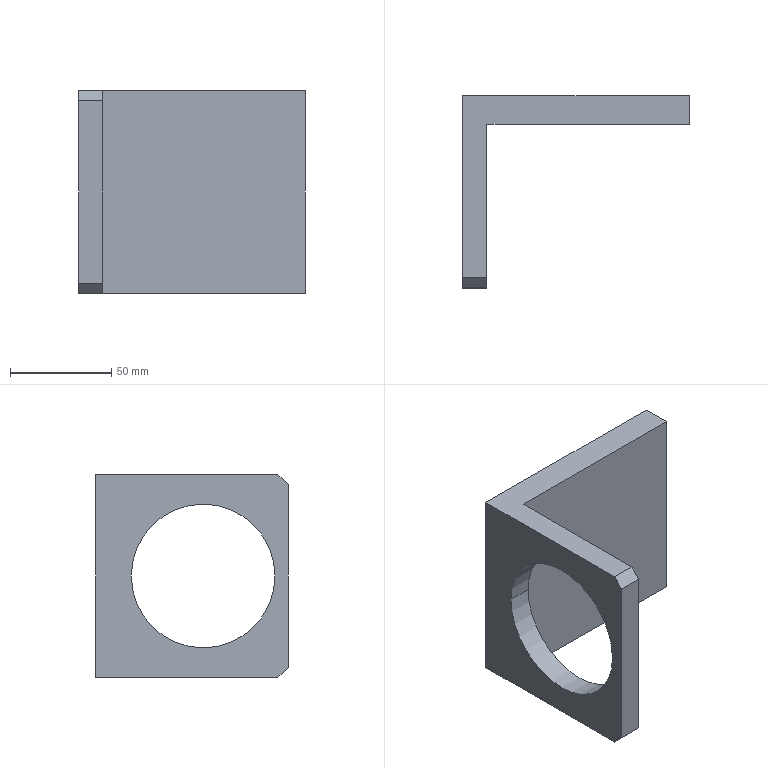Part | SolidWorks | features ICE 2, Chamfer 1, Extrusion 1 | 1 solid | 12 faces | box 112 x 95 x 100 mm | volume 206190 mm3 | plane 10 | cylinder 2 | commonest cylinder face diameters 71 x2
STEP:
#1=CARTESIAN_POINT('',(0.,77.5,0.));
#2=VERTEX_POINT('',#1);
#3=CARTESIAN_POINT('',(0.,6.5,0.));
#4=VERTEX_POINT('',#3);
#5=CARTESIAN_POINT('',(0.,42.,0.));
#6=DIRECTION('',(-1.,0.,0.));
#7=DIRECTION('',(0.,0.,-1.));
#8=AXIS2_PLACEMENT_3D('',#5,#6,#7);
#9=CIRCLE('',#8,35.5);
#10=EDGE_CURVE('',#2,#4,#9,.T.);
#11=ORIENTED_EDGE('',*,*,#10,.T.);
#12=CARTESIAN_POINT('',(12.,6.5,0.));
#13=VERTEX_POINT('',#12);
#14=CARTESIAN_POINT('',(-0.001,6.5,0.));
#15=DIRECTION('',(1.,0.,0.));
#16=VECTOR('',#15,1000.);
#17=LINE('',#14,#16);
#18=EDGE_CURVE('',#4,#13,#17,.T.);
#19=ORIENTED_EDGE('',*,*,#18,.T.);
#20=CARTESIAN_POINT('',(12.,77.5,0.));
#21=VERTEX_POINT('',#20);
#22=CARTESIAN_POINT('',(12.,42.,0.));
#23=DIRECTION('',(1.,0.,0.));
#24=DIRECTION('',(0.,1.,0.));
#25=AXIS2_PLACEMENT_3D('',#22,#23,#24);
#26=CIRCLE('',#25,35.5);
#27=EDGE_CURVE('',#13,#21,#26,.T.);
#28=ORIENTED_EDGE('',*,*,#27,.T.);
#29=CARTESIAN_POINT('',(-0.001,77.5,0.));
#30=DIRECTION('',(1.,0.,0.));
#31=VECTOR('',#30,1000.);
#32=LINE('',#29,#31);
#33=EDGE_CURVE('',#2,#21,#32,.T.);
#34=ORIENTED_EDGE('',*,*,#33,.F.);
#35=EDGE_LOOP('',(#11,#19,#28,#34));
#36=FACE_OUTER_BOUND('',#35,.T.);
#37=CARTESIAN_POINT('',(-0.001,42.,0.));
#38=DIRECTION('',(1.,0.,0.));
#39=DIRECTION('',(0.,1.,0.));
#40=AXIS2_PLACEMENT_3D('',#37,#38,#39);
#41=CYLINDRICAL_SURFACE('',#40,35.5);
#42=ADVANCED_FACE('',(#36),#41,.F.);
#43=CARTESIAN_POINT('',(12.,42.,0.));
#44=DIRECTION('',(1.,0.,0.));
#45=DIRECTION('',(0.,1.,0.));
#46=AXIS2_PLACEMENT_3D('',#43,#44,#45);
#47=CIRCLE('',#46,35.5);
#48=EDGE_CURVE('',#21,#13,#47,.T.);
#49=ORIENTED_EDGE('',*,*,#48,.F.);
#50=ORIENTED_EDGE('',*,*,#27,.F.);
#51=EDGE_LOOP('',(#49,#50));
#52=FACE_BOUND('',#51,.T.);
#53=CARTESIAN_POINT('',(12.,5.,50.));
#54=VERTEX_POINT('',#53);
#55=CARTESIAN_POINT('',(12.,81.,50.));
#56=VERTEX_POINT('',#55);
#57=CARTESIAN_POINT('',(12.,95.,50.));
#58=DIRECTION('',(0.,1.,0.));
#59=VECTOR('',#58,1000.);
#60=LINE('',#57,#59);
#61=EDGE_CURVE('',#54,#56,#60,.T.);
#62=ORIENTED_EDGE('',*,*,#61,.F.);
#63=CARTESIAN_POINT('',(12.,0.,45.));
#64=VERTEX_POINT('',#63);
#65=CARTESIAN_POINT('',(12.,5.,50.));
#66=DIRECTION('',(0.,-0.7071,-0.7071));
#67=VECTOR('',#66,1000.);
#68=LINE('',#65,#67);
#69=EDGE_CURVE('',#54,#64,#68,.T.);
#70=ORIENTED_EDGE('',*,*,#69,.T.);
#71=CARTESIAN_POINT('',(12.,0.,-45.));
#72=VERTEX_POINT('',#71);
#73=CARTESIAN_POINT('',(12.,0.,50.));
#74=DIRECTION('',(0.,0.,-1.));
#75=VECTOR('',#74,1000.);
#76=LINE('',#73,#75);
#77=EDGE_CURVE('',#64,#72,#76,.T.);
#78=ORIENTED_EDGE('',*,*,#77,.T.);
#79=CARTESIAN_POINT('',(12.,5.,-50.));
#80=VERTEX_POINT('',#79);
#81=CARTESIAN_POINT('',(12.,0.,-45.));
#82=DIRECTION('',(0.,0.7071,-0.7071));
#83=VECTOR('',#82,1000.);
#84=LINE('',#81,#83);
#85=EDGE_CURVE('',#72,#80,#84,.T.);
#86=ORIENTED_EDGE('',*,*,#85,.T.);
#87=CARTESIAN_POINT('',(12.,81.,-50.));
#88=VERTEX_POINT('',#87);
#89=CARTESIAN_POINT('',(12.,95.,-50.));
#90=DIRECTION('',(0.,1.,0.));
#91=VECTOR('',#90,1000.);
#92=LINE('',#89,#91);
#93=EDGE_CURVE('',#80,#88,#92,.T.);
#94=ORIENTED_EDGE('',*,*,#93,.T.);
#95=CARTESIAN_POINT('',(12.,81.,50.));
#96=DIRECTION('',(0.,0.,-1.));
#97=VECTOR('',#96,1000.);
#98=LINE('',#95,#97);
#99=EDGE_CURVE('',#56,#88,#98,.T.);
#100=ORIENTED_EDGE('',*,*,#99,.F.);
#101=EDGE_LOOP('',(#62,#70,#78,#86,#94,#100));
#102=FACE_OUTER_BOUND('',#101,.T.);
#103=CARTESIAN_POINT('',(12.,95.,50.));
#104=DIRECTION('',(-1.,0.,0.));
#105=DIRECTION('',(0.,-1.,0.));
#106=AXIS2_PLACEMENT_3D('',#103,#104,#105);
#107=PLANE('',#106);
#108=ADVANCED_FACE('',(#52,#102),#107,.F.);
#109=ORIENTED_EDGE('',*,*,#77,.F.);
#110=CARTESIAN_POINT('',(0.,0.,45.));
#111=VERTEX_POINT('',#110);
#112=CARTESIAN_POINT('',(12.,0.,45.));
#113=DIRECTION('',(-1.,0.,0.));
#114=VECTOR('',#113,1000.);
#115=LINE('',#112,#114);
#116=EDGE_CURVE('',#64,#111,#115,.T.);
#117=ORIENTED_EDGE('',*,*,#116,.T.);
#118=CARTESIAN_POINT('',(0.,0.,-45.));
#119=VERTEX_POINT('',#118);
#120=CARTESIAN_POINT('',(0.,0.,50.));
#121=DIRECTION('',(0.,0.,-1.));
#122=VECTOR('',#121,1000.);
#123=LINE('',#120,#122);
#124=EDGE_CURVE('',#111,#119,#123,.T.);
#125=ORIENTED_EDGE('',*,*,#124,.T.);
#126=CARTESIAN_POINT('',(12.,0.,-45.));
#127=DIRECTION('',(1.,0.,0.));
#128=VECTOR('',#127,1000.);
#129=LINE('',#126,#128);
#130=EDGE_CURVE('',#119,#72,#129,.T.);
#131=ORIENTED_EDGE('',*,*,#130,.T.);
#132=EDGE_LOOP('',(#109,#117,#125,#131));
#133=FACE_OUTER_BOUND('',#132,.T.);
#134=CARTESIAN_POINT('',(12.,0.,50.));
#135=DIRECTION('',(0.,1.,0.));
#136=DIRECTION('',(0.,0.,1.));
#137=AXIS2_PLACEMENT_3D('',#134,#135,#136);
#138=PLANE('',#137);
#139=ADVANCED_FACE('',(#133),#138,.F.);
#140=CARTESIAN_POINT('',(112.,95.,-50.));
#141=VERTEX_POINT('',#140);
#142=CARTESIAN_POINT('',(0.,95.,-50.));
#143=VERTEX_POINT('',#142);
#144=CARTESIAN_POINT('',(12.,95.,-50.));
#145=DIRECTION('',(-1.,0.,0.));
#146=VECTOR('',#145,1000.);
#147=LINE('',#144,#146);
#148=EDGE_CURVE('',#141,#143,#147,.T.);
#149=ORIENTED_EDGE('',*,*,#148,.T.);
#150=CARTESIAN_POINT('',(0.,95.,50.));
#151=VERTEX_POINT('',#150);
#152=CARTESIAN_POINT('',(0.,95.,50.));
#153=DIRECTION('',(0.,0.,-1.));
#154=VECTOR('',#153,1000.);
#155=LINE('',#152,#154);
#156=EDGE_CURVE('',#151,#143,#155,.T.);
#157=ORIENTED_EDGE('',*,*,#156,.F.);
#158=CARTESIAN_POINT('',(112.,95.,50.));
#159=VERTEX_POINT('',#158);
#160=CARTESIAN_POINT('',(12.,95.,50.));
#161=DIRECTION('',(-1.,0.,0.));
#162=VECTOR('',#161,1000.);
#163=LINE('',#160,#162);
#164=EDGE_CURVE('',#159,#151,#163,.T.);
#165=ORIENTED_EDGE('',*,*,#164,.F.);
#166=CARTESIAN_POINT('',(112.,95.,50.));
#167=DIRECTION('',(0.,0.,1.));
#168=VECTOR('',#167,1000.);
#169=LINE('',#166,#168);
#170=EDGE_CURVE('',#141,#159,#169,.T.);
#171=ORIENTED_EDGE('',*,*,#170,.F.);
#172=EDGE_LOOP('',(#149,#157,#165,#171));
#173=FACE_OUTER_BOUND('',#172,.T.);
#174=CARTESIAN_POINT('',(12.,95.,50.));
#175=DIRECTION('',(0.,-1.,0.));
#176=DIRECTION('',(0.,0.,-1.));
#177=AXIS2_PLACEMENT_3D('',#174,#175,#176);
#178=PLANE('',#177);
#179=ADVANCED_FACE('',(#173),#178,.F.);
#180=ORIENTED_EDGE('',*,*,#10,.F.);
#181=CARTESIAN_POINT('',(0.,42.,0.));
#182=DIRECTION('',(-1.,0.,0.));
#183=DIRECTION('',(0.,0.,-1.));
#184=AXIS2_PLACEMENT_3D('',#181,#182,#183);
#185=CIRCLE('',#184,35.5);
#186=EDGE_CURVE('',#4,#2,#185,.T.);
#187=ORIENTED_EDGE('',*,*,#186,.F.);
#188=EDGE_LOOP('',(#180,#187));
#189=FACE_BOUND('',#188,.T.);
#190=ORIENTED_EDGE('',*,*,#124,.F.);
#191=CARTESIAN_POINT('',(0.,5.,50.));
#192=VERTEX_POINT('',#191);
#193=CARTESIAN_POINT('',(0.,5.,50.));
#194=DIRECTION('',(0.,0.7071,0.7071));
#195=VECTOR('',#194,1000.);
#196=LINE('',#193,#195);
#197=EDGE_CURVE('',#111,#192,#196,.T.);
#198=ORIENTED_EDGE('',*,*,#197,.T.);
#199=CARTESIAN_POINT('',(0.,0.,50.));
#200=DIRECTION('',(0.,-1.,0.));
#201=VECTOR('',#200,1000.);
#202=LINE('',#199,#201);
#203=EDGE_CURVE('',#151,#192,#202,.T.);
#204=ORIENTED_EDGE('',*,*,#203,.F.);
#205=ORIENTED_EDGE('',*,*,#156,.T.);
#206=CARTESIAN_POINT('',(0.,5.,-50.));
#207=VERTEX_POINT('',#206);
#208=CARTESIAN_POINT('',(0.,0.,-50.));
#209=DIRECTION('',(0.,-1.,0.));
#210=VECTOR('',#209,1000.);
#211=LINE('',#208,#210);
#212=EDGE_CURVE('',#143,#207,#211,.T.);
#213=ORIENTED_EDGE('',*,*,#212,.T.);
#214=CARTESIAN_POINT('',(0.,0.,-45.));
#215=DIRECTION('',(0.,-0.7071,0.7071));
#216=VECTOR('',#215,1000.);
#217=LINE('',#214,#216);
#218=EDGE_CURVE('',#207,#119,#217,.T.);
#219=ORIENTED_EDGE('',*,*,#218,.T.);
#220=EDGE_LOOP('',(#190,#198,#204,#205,#213,#219));
#221=FACE_OUTER_BOUND('',#220,.T.);
#222=CARTESIAN_POINT('',(0.,0.,50.));
#223=DIRECTION('',(1.,0.,0.));
#224=DIRECTION('',(0.,0.,-1.));
#225=AXIS2_PLACEMENT_3D('',#222,#223,#224);
#226=PLANE('',#225);
#227=ADVANCED_FACE('',(#189,#221),#226,.F.);
#228=ORIENTED_EDGE('',*,*,#203,.T.);
#229=CARTESIAN_POINT('',(0.,5.,50.));
#230=DIRECTION('',(1.,0.,0.));
#231=VECTOR('',#230,1000.);
#232=LINE('',#229,#231);
#233=EDGE_CURVE('',#192,#54,#232,.T.);
#234=ORIENTED_EDGE('',*,*,#233,.T.);
#235=ORIENTED_EDGE('',*,*,#61,.T.);
#236=CARTESIAN_POINT('',(112.,81.,50.));
#237=VERTEX_POINT('',#236);
#238=CARTESIAN_POINT('',(112.,81.,50.));
#239=DIRECTION('',(-1.,0.,0.));
#240=VECTOR('',#239,1000.);
#241=LINE('',#238,#240);
#242=EDGE_CURVE('',#237,#56,#241,.T.);
#243=ORIENTED_EDGE('',*,*,#242,.F.);
#244=CARTESIAN_POINT('',(112.,95.,50.));
#245=DIRECTION('',(0.,-1.,0.));
#246=VECTOR('',#245,1000.);
#247=LINE('',#244,#246);
#248=EDGE_CURVE('',#159,#237,#247,.T.);
#249=ORIENTED_EDGE('',*,*,#248,.F.);
#250=ORIENTED_EDGE('',*,*,#164,.T.);
#251=EDGE_LOOP('',(#228,#234,#235,#243,#249,#250));
#252=FACE_OUTER_BOUND('',#251,.T.);
#253=CARTESIAN_POINT('',(0.,0.,50.));
#254=DIRECTION('',(0.,0.,-1.));
#255=DIRECTION('',(-1.,0.,0.));
#256=AXIS2_PLACEMENT_3D('',#253,#254,#255);
#257=PLANE('',#256);
#258=ADVANCED_FACE('',(#252),#257,.F.);
#259=ORIENTED_EDGE('',*,*,#93,.F.);
#260=CARTESIAN_POINT('',(0.,5.,-50.));
#261=DIRECTION('',(-1.,0.,0.));
#262=VECTOR('',#261,1000.);
#263=LINE('',#260,#262);
#264=EDGE_CURVE('',#80,#207,#263,.T.);
#265=ORIENTED_EDGE('',*,*,#264,.T.);
#266=ORIENTED_EDGE('',*,*,#212,.F.);
#267=ORIENTED_EDGE('',*,*,#148,.F.);
#268=CARTESIAN_POINT('',(112.,81.,-50.));
#269=VERTEX_POINT('',#268);
#270=CARTESIAN_POINT('',(112.,95.,-50.));
#271=DIRECTION('',(0.,1.,0.));
#272=VECTOR('',#271,1000.);
#273=LINE('',#270,#272);
#274=EDGE_CURVE('',#269,#141,#273,.T.);
#275=ORIENTED_EDGE('',*,*,#274,.F.);
#276=CARTESIAN_POINT('',(112.,81.,-50.));
#277=DIRECTION('',(-1.,0.,0.));
#278=VECTOR('',#277,1000.);
#279=LINE('',#276,#278);
#280=EDGE_CURVE('',#269,#88,#279,.T.);
#281=ORIENTED_EDGE('',*,*,#280,.T.);
#282=EDGE_LOOP('',(#259,#265,#266,#267,#275,#281));
#283=FACE_OUTER_BOUND('',#282,.T.);
#284=CARTESIAN_POINT('',(0.,0.,-50.));
#285=DIRECTION('',(0.,0.,-1.));
#286=DIRECTION('',(-1.,0.,0.));
#287=AXIS2_PLACEMENT_3D('',#284,#285,#286);
#288=PLANE('',#287);
#289=ADVANCED_FACE('',(#283),#288,.T.);
#290=ORIENTED_EDGE('',*,*,#18,.F.);
#291=ORIENTED_EDGE('',*,*,#186,.T.);
#292=ORIENTED_EDGE('',*,*,#33,.T.);
#293=ORIENTED_EDGE('',*,*,#48,.T.);
#294=EDGE_LOOP('',(#290,#291,#292,#293));
#295=FACE_OUTER_BOUND('',#294,.T.);
#296=CARTESIAN_POINT('',(-0.001,42.,0.));
#297=DIRECTION('',(1.,0.,0.));
#298=DIRECTION('',(0.,1.,0.));
#299=AXIS2_PLACEMENT_3D('',#296,#297,#298);
#300=CYLINDRICAL_SURFACE('',#299,35.5);
#301=ADVANCED_FACE('',(#295),#300,.F.);
#302=ORIENTED_EDGE('',*,*,#99,.T.);
#303=ORIENTED_EDGE('',*,*,#280,.F.);
#304=CARTESIAN_POINT('',(112.,81.,50.));
#305=DIRECTION('',(0.,0.,-1.));
#306=VECTOR('',#305,1000.);
#307=LINE('',#304,#306);
#308=EDGE_CURVE('',#237,#269,#307,.T.);
#309=ORIENTED_EDGE('',*,*,#308,.F.);
#310=ORIENTED_EDGE('',*,*,#242,.T.);
#311=EDGE_LOOP('',(#302,#303,#309,#310));
#312=FACE_OUTER_BOUND('',#311,.T.);
#313=CARTESIAN_POINT('',(112.,81.,50.));
#314=DIRECTION('',(0.,1.,0.));
#315=DIRECTION('',(-1.,0.,0.));
#316=AXIS2_PLACEMENT_3D('',#313,#314,#315);
#317=PLANE('',#316);
#318=ADVANCED_FACE('',(#312),#317,.F.);
#319=ORIENTED_EDGE('',*,*,#248,.T.);
#320=ORIENTED_EDGE('',*,*,#308,.T.);
#321=ORIENTED_EDGE('',*,*,#274,.T.);
#322=ORIENTED_EDGE('',*,*,#170,.T.);
#323=EDGE_LOOP('',(#319,#320,#321,#322));
#324=FACE_OUTER_BOUND('',#323,.T.);
#325=CARTESIAN_POINT('',(112.,0.,0.));
#326=DIRECTION('',(1.,0.,0.));
#327=DIRECTION('',(0.,1.,0.));
#328=AXIS2_PLACEMENT_3D('',#325,#326,#327);
#329=PLANE('',#328);
#330=ADVANCED_FACE('',(#324),#329,.T.);
#331=ORIENTED_EDGE('',*,*,#197,.F.);
#332=ORIENTED_EDGE('',*,*,#116,.F.);
#333=ORIENTED_EDGE('',*,*,#69,.F.);
#334=ORIENTED_EDGE('',*,*,#233,.F.);
#335=EDGE_LOOP('',(#331,#332,#333,#334));
#336=FACE_OUTER_BOUND('',#335,.T.);
#337=CARTESIAN_POINT('',(0.,5.,50.));
#338=DIRECTION('',(0.,0.7071,-0.7071));
#339=DIRECTION('',(1.,0.,0.));
#340=AXIS2_PLACEMENT_3D('',#337,#338,#339);
#341=PLANE('',#340);
#342=ADVANCED_FACE('',(#336),#341,.F.);
#343=ORIENTED_EDGE('',*,*,#218,.F.);
#344=ORIENTED_EDGE('',*,*,#264,.F.);
#345=ORIENTED_EDGE('',*,*,#85,.F.);
#346=ORIENTED_EDGE('',*,*,#130,.F.);
#347=EDGE_LOOP('',(#343,#344,#345,#346));
#348=FACE_OUTER_BOUND('',#347,.T.);
#349=CARTESIAN_POINT('',(12.,0.,-45.));
#350=DIRECTION('',(0.,-0.7071,-0.7071));
#351=DIRECTION('',(-1.,0.,0.));
#352=AXIS2_PLACEMENT_3D('',#349,#350,#351);
#353=PLANE('',#352);
#354=ADVANCED_FACE('',(#348),#353,.T.);
#355=CLOSED_SHELL('',(#42,#108,#139,#179,#227,#258,#289,#301,#318,#330,#342,#354));
#356=MANIFOLD_SOLID_BREP('',#355);
#357=CARTESIAN_POINT('',(0.,0.,0.));
#358=DIRECTION('',(0.,0.,1.));
#359=DIRECTION('',(1.,0.,0.));
#360=AXIS2_PLACEMENT_3D('',#357,#358,#359);
#361=(LENGTH_UNIT()NAMED_UNIT(*)SI_UNIT(.MILLI.,.METRE.));
#362=UNCERTAINTY_MEASURE_WITH_UNIT(LENGTH_MEASURE(0.00001),#361,'','');
#363=(NAMED_UNIT(*)PLANE_ANGLE_UNIT()SI_UNIT($,.RADIAN.));
#364=(NAMED_UNIT(*)SI_UNIT($,.STERADIAN.)SOLID_ANGLE_UNIT());
#365=(GEOMETRIC_REPRESENTATION_CONTEXT(3)GLOBAL_UNCERTAINTY_ASSIGNED_CONTEXT((#362))GLOBAL_UNIT_ASSIGNED_CONTEXT((#361,#363,#364))REPRESENTATION_CONTEXT('',''));
#366=ADVANCED_BREP_SHAPE_REPRESENTATION('',(#356,#360),#365);